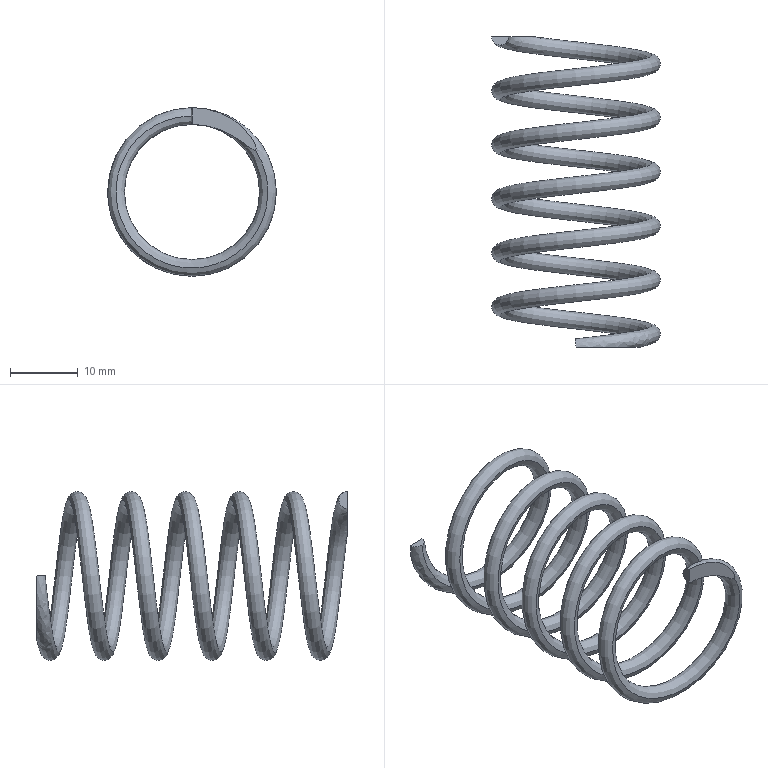Part | SolidWorks | features Helix 2, ICE 2, Sweep 2 | 1 solid | 6 faces | box 25 x 46 x 25 mm | volume 1991 mm3 | plane 4 | spline 2